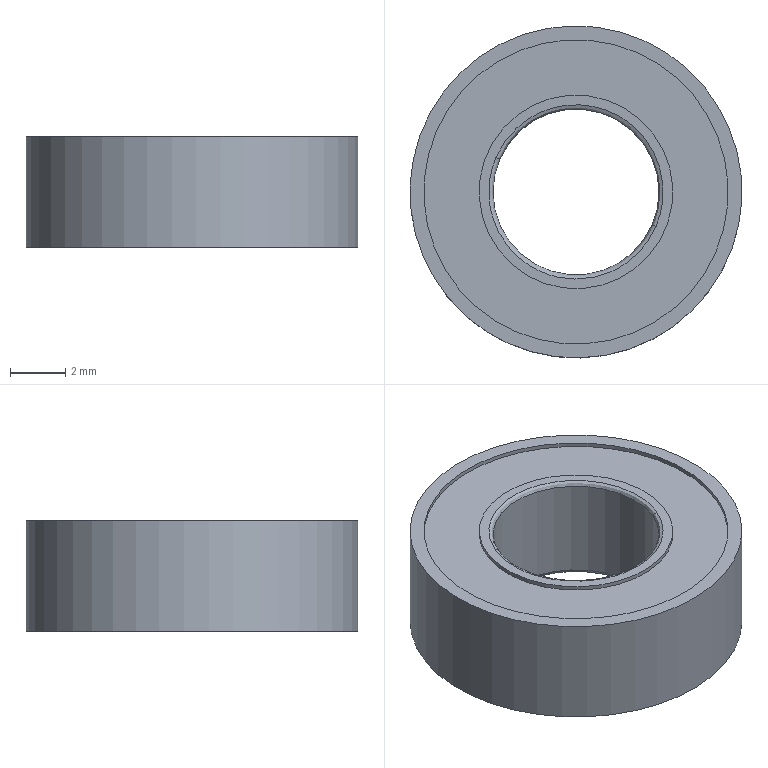Part | STEP file | Zapas-OpenRC Truggy HSPr v2. v55-1 | 1 solid | 16 faces | box 12 x 12 x 4 mm | volume 322.133 mm3 | cylinder 6 | plane 6 | spline 4 | commonest cylinder face diameters 7 x2 11 x2 6 x1 12 x1